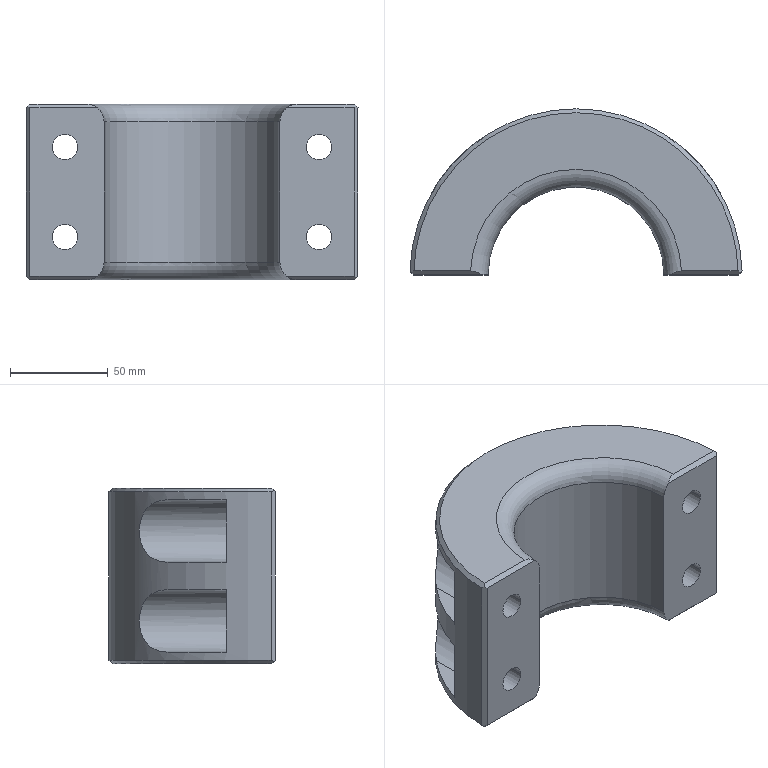Part | Creo | features DATUM PLANE 4, CURVE 3, CUT 2, CHAMFER 1, COORDINATE SYSTEM 1, PROTRUSION 1, ROUND 1 | 1 solid | 40 faces | box 170 x 85 x 90 mm | volume 620159 mm3 | plane 22 | cylinder 14 | torus 2 | cone 2 | commonest cylinder face diameters 13 x8 32 x4 90 x1 170 x1
STEP:
#1=CARTESIAN_POINT('',(0.,0.,0.));
#2=DIRECTION('',(0.,0.,1.));
#3=DIRECTION('',(1.,0.,0.));
#4=AXIS2_PLACEMENT_3D('',#1,#2,#3);
#5=CARTESIAN_POINT('',(53.963,2.,-45.));
#6=VERTEX_POINT('',#5);
#7=CARTESIAN_POINT('',(-53.963,2.,-45.));
#8=VERTEX_POINT('',#7);
#9=CARTESIAN_POINT('',(0.,0.,-45.));
#10=DIRECTION('',(0.,0.,1.));
#11=DIRECTION('',(0.9993,0.03704,0.));
#12=AXIS2_PLACEMENT_3D('',#9,#10,#11);
#13=CIRCLE('',#12,54.);
#14=EDGE_CURVE('',#6,#8,#13,.T.);
#15=ORIENTED_EDGE('',*,*,#14,.F.);
#16=CARTESIAN_POINT('',(82.976,2.,-45.));
#17=VERTEX_POINT('',#16);
#18=CARTESIAN_POINT('',(82.976,2.,-45.));
#19=DIRECTION('',(-1.,0.,-0.000000001));
#20=VECTOR('',#19,29.013);
#21=LINE('',#18,#20);
#22=EDGE_CURVE('',#17,#6,#21,.T.);
#23=ORIENTED_EDGE('',*,*,#22,.F.);
#24=CARTESIAN_POINT('',(-82.976,2.,-45.));
#25=VERTEX_POINT('',#24);
#26=CARTESIAN_POINT('',(-0.00000004,0.000000008,-45.));
#27=DIRECTION('',(0.,0.,-1.));
#28=DIRECTION('',(-0.9997,0.0241,0.));
#29=AXIS2_PLACEMENT_3D('',#26,#27,#28);
#30=CIRCLE('',#29,83.);
#31=EDGE_CURVE('',#25,#17,#30,.T.);
#32=ORIENTED_EDGE('',*,*,#31,.F.);
#33=CARTESIAN_POINT('',(-53.963,2.,-45.));
#34=DIRECTION('',(-1.,0.,0.));
#35=VECTOR('',#34,29.013);
#36=LINE('',#33,#35);
#37=EDGE_CURVE('',#8,#25,#36,.T.);
#38=ORIENTED_EDGE('',*,*,#37,.F.);
#39=EDGE_LOOP('',(#15,#23,#32,#38));
#40=FACE_OUTER_BOUND('',#39,.F.);
#41=CARTESIAN_POINT('',(0.,0.,-45.));
#42=DIRECTION('',(0.,0.,1.));
#43=DIRECTION('',(1.,0.,0.));
#44=AXIS2_PLACEMENT_3D('',#41,#42,#43);
#45=PLANE('',#44);
#46=ADVANCED_FACE('',(#40),#45,.F.);
#47=ORIENTED_EDGE('',*,*,#14,.T.);
#48=CARTESIAN_POINT('',(-48.343,0.,-43.));
#49=VERTEX_POINT('',#48);
#50=CARTESIAN_POINT('',(-53.546,2.,-45.));
#51=CARTESIAN_POINT('',(-52.717,1.945,-44.945));
#52=CARTESIAN_POINT('',(-51.42,1.663,-44.663));
#53=CARTESIAN_POINT('',(-50.257,1.222,-44.222));
#54=CARTESIAN_POINT('',(-49.214,0.653,-43.653));
#55=CARTESIAN_POINT('',(-48.622,0.2252,-43.225));
#56=B_SPLINE_CURVE_WITH_KNOTS('',3,(#7,#50,#51,#52,#53,#54,#55,#48),.UNSPECIFIED.,.F.,.F.,(4,1,1,1,1,4),(0.,0.2,0.4,0.6,0.8,1.),.UNSPECIFIED.);
#57=EDGE_CURVE('',#8,#49,#56,.T.);
#58=ORIENTED_EDGE('',*,*,#57,.T.);
#59=CARTESIAN_POINT('',(-45.,0.,-36.));
#60=VERTEX_POINT('',#59);
#61=CARTESIAN_POINT('',(-54.,0.,-36.));
#62=DIRECTION('',(0.,-1.,0.));
#63=DIRECTION('',(0.6285,0.,-0.7778));
#64=AXIS2_PLACEMENT_3D('',#61,#62,#63);
#65=CIRCLE('',#64,9.);
#66=EDGE_CURVE('',#49,#60,#65,.T.);
#67=ORIENTED_EDGE('',*,*,#66,.T.);
#68=CARTESIAN_POINT('',(45.,0.,-36.));
#69=VERTEX_POINT('',#68);
#70=CARTESIAN_POINT('',(0.,0.,-36.));
#71=DIRECTION('',(0.,0.,-1.));
#72=DIRECTION('',(-1.,0.,0.));
#73=AXIS2_PLACEMENT_3D('',#70,#71,#72);
#74=CIRCLE('',#73,45.);
#75=EDGE_CURVE('',#60,#69,#74,.T.);
#76=ORIENTED_EDGE('',*,*,#75,.T.);
#77=CARTESIAN_POINT('',(48.343,0.,-43.));
#78=VERTEX_POINT('',#77);
#79=CARTESIAN_POINT('',(54.,0.,-36.));
#80=DIRECTION('',(0.,-1.,0.));
#81=DIRECTION('',(-1.,0.,0.));
#82=AXIS2_PLACEMENT_3D('',#79,#80,#81);
#83=CIRCLE('',#82,9.);
#84=EDGE_CURVE('',#69,#78,#83,.T.);
#85=ORIENTED_EDGE('',*,*,#84,.T.);
#86=CARTESIAN_POINT('',(48.343,0.,-43.));
#87=CARTESIAN_POINT('',(48.622,0.2255,-43.226));
#88=CARTESIAN_POINT('',(49.215,0.6537,-43.654));
#89=CARTESIAN_POINT('',(50.258,1.222,-44.222));
#90=CARTESIAN_POINT('',(51.421,1.663,-44.663));
#91=CARTESIAN_POINT('',(52.717,1.945,-44.945));
#92=CARTESIAN_POINT('',(53.546,2.,-45.));
#93=B_SPLINE_CURVE_WITH_KNOTS('',3,(#86,#87,#88,#89,#90,#91,#92,#5),.UNSPECIFIED.,.F.,.F.,(4,1,1,1,1,4),(0.,0.2,0.4,0.6,0.8,1.),.UNSPECIFIED.);
#94=EDGE_CURVE('',#78,#6,#93,.T.);
#95=ORIENTED_EDGE('',*,*,#94,.T.);
#96=EDGE_LOOP('',(#47,#58,#67,#76,#85,#95));
#97=FACE_OUTER_BOUND('',#96,.F.);
#98=CARTESIAN_POINT('',(0.,0.,-36.));
#99=DIRECTION('',(0.,0.,1.));
#100=DIRECTION('',(0.001486,-1.,0.));
#101=AXIS2_PLACEMENT_3D('',#98,#99,#100);
#102=TOROIDAL_SURFACE('',#101,54.,9.);
#103=ADVANCED_FACE('',(#97),#102,.T.);
#104=ORIENTED_EDGE('',*,*,#57,.F.);
#105=ORIENTED_EDGE('',*,*,#37,.T.);
#106=CARTESIAN_POINT('',(-83.973,1.021,-44.021));
#107=VERTEX_POINT('',#106);
#108=CARTESIAN_POINT('',(-83.086,1.892,-44.892));
#109=CARTESIAN_POINT('',(-83.308,1.676,-44.676));
#110=CARTESIAN_POINT('',(-83.64,1.35,-44.35));
#111=CARTESIAN_POINT('',(-83.862,1.131,-44.131));
#112=CARTESIAN_POINT('',(-83.973,1.021,-44.021));
#113=B_SPLINE_CURVE_WITH_KNOTS('',3,(#24,#108,#109,#110,#111,#112),.UNSPECIFIED.,.F.,.F.,(4,1,1,4),(0.,0.3333,0.6667,1.),.UNSPECIFIED.);
#114=EDGE_CURVE('',#25,#107,#113,.T.);
#115=ORIENTED_EDGE('',*,*,#114,.T.);
#116=CARTESIAN_POINT('',(-82.976,0.,-43.));
#117=VERTEX_POINT('',#116);
#118=CARTESIAN_POINT('',(-83.973,1.021,-44.021));
#119=DIRECTION('',(0.5681,-0.5819,0.5819));
#120=VECTOR('',#119,1.755);
#121=LINE('',#118,#120);
#122=EDGE_CURVE('',#107,#117,#121,.T.);
#123=ORIENTED_EDGE('',*,*,#122,.T.);
#124=CARTESIAN_POINT('',(-48.343,0.,-43.));
#125=DIRECTION('',(-1.,0.,0.));
#126=VECTOR('',#125,34.633);
#127=LINE('',#124,#126);
#128=EDGE_CURVE('',#49,#117,#127,.T.);
#129=ORIENTED_EDGE('',*,*,#128,.F.);
#130=EDGE_LOOP('',(#104,#105,#115,#123,#129));
#131=FACE_OUTER_BOUND('',#130,.F.);
#132=CARTESIAN_POINT('',(-64.988,1.,-44.));
#133=DIRECTION('',(0.,-0.7071,-0.7071));
#134=DIRECTION('',(0.,-0.7071,0.7071));
#135=AXIS2_PLACEMENT_3D('',#132,#133,#134);
#136=PLANE('',#135);
#137=ADVANCED_FACE('',(#131),#136,.T.);
#138=ORIENTED_EDGE('',*,*,#31,.T.);
#139=CARTESIAN_POINT('',(83.973,1.021,-44.021));
#140=VERTEX_POINT('',#139);
#141=CARTESIAN_POINT('',(83.973,1.021,-44.021));
#142=CARTESIAN_POINT('',(83.862,1.131,-44.131));
#143=CARTESIAN_POINT('',(83.64,1.35,-44.35));
#144=CARTESIAN_POINT('',(83.308,1.676,-44.676));
#145=CARTESIAN_POINT('',(83.086,1.892,-44.892));
#146=B_SPLINE_CURVE_WITH_KNOTS('',3,(#141,#142,#143,#144,#145,#16),.UNSPECIFIED.,.F.,.F.,(4,1,1,4),(0.,0.3333,0.6667,1.),.UNSPECIFIED.);
#147=EDGE_CURVE('',#140,#17,#146,.T.);
#148=ORIENTED_EDGE('',*,*,#147,.F.);
#149=CARTESIAN_POINT('',(84.975,2.048,-43.));
#150=VERTEX_POINT('',#149);
#151=CARTESIAN_POINT('',(84.975,2.048,-43.));
#152=CARTESIAN_POINT('',(84.863,1.933,-43.115));
#153=CARTESIAN_POINT('',(84.639,1.704,-43.344));
#154=CARTESIAN_POINT('',(84.305,1.361,-43.684));
#155=CARTESIAN_POINT('',(84.083,1.134,-43.909));
#156=B_SPLINE_CURVE_WITH_KNOTS('',3,(#151,#152,#153,#154,#155,#139),.UNSPECIFIED.,.F.,.F.,(4,1,1,4),(0.,0.3333,0.6667,1.),.UNSPECIFIED.);
#157=EDGE_CURVE('',#150,#140,#156,.T.);
#158=ORIENTED_EDGE('',*,*,#157,.F.);
#159=CARTESIAN_POINT('',(-84.975,2.048,-43.));
#160=VERTEX_POINT('',#159);
#161=CARTESIAN_POINT('',(-0.00000004,0.000000008,-43.));
#162=DIRECTION('',(0.,0.,1.));
#163=DIRECTION('',(0.9997,0.0241,0.));
#164=AXIS2_PLACEMENT_3D('',#161,#162,#163);
#165=CIRCLE('',#164,85.);
#166=EDGE_CURVE('',#150,#160,#165,.T.);
#167=ORIENTED_EDGE('',*,*,#166,.T.);
#168=CARTESIAN_POINT('',(-84.975,2.048,-43.));
#169=CARTESIAN_POINT('',(-84.863,1.933,-43.115));
#170=CARTESIAN_POINT('',(-84.639,1.704,-43.344));
#171=CARTESIAN_POINT('',(-84.305,1.361,-43.684));
#172=CARTESIAN_POINT('',(-84.083,1.134,-43.909));
#173=B_SPLINE_CURVE_WITH_KNOTS('',3,(#168,#169,#170,#171,#172,#106),.UNSPECIFIED.,.F.,.F.,(4,1,1,4),(0.,0.3333,0.6667,1.),.UNSPECIFIED.);
#174=EDGE_CURVE('',#160,#107,#173,.T.);
#175=ORIENTED_EDGE('',*,*,#174,.T.);
#176=ORIENTED_EDGE('',*,*,#114,.F.);
#177=EDGE_LOOP('',(#138,#148,#158,#167,#175,#176));
#178=FACE_OUTER_BOUND('',#177,.F.);
#179=CARTESIAN_POINT('',(-0.00000004,0.000000008,-44.));
#180=DIRECTION('',(0.,0.,1.));
#181=DIRECTION('',(0.,-1.,0.));
#182=AXIS2_PLACEMENT_3D('',#179,#180,#181);
#183=CONICAL_SURFACE('',#182,84.,45.);
#184=ADVANCED_FACE('',(#178),#183,.T.);
#185=ORIENTED_EDGE('',*,*,#94,.F.);
#186=CARTESIAN_POINT('',(82.976,0.,-43.));
#187=VERTEX_POINT('',#186);
#188=CARTESIAN_POINT('',(82.976,0.,-43.));
#189=DIRECTION('',(-1.,0.,0.));
#190=VECTOR('',#189,34.633);
#191=LINE('',#188,#190);
#192=EDGE_CURVE('',#187,#78,#191,.T.);
#193=ORIENTED_EDGE('',*,*,#192,.F.);
#194=CARTESIAN_POINT('',(82.976,0.,-43.));
#195=DIRECTION('',(0.5681,0.5819,-0.5819));
#196=VECTOR('',#195,1.755);
#197=LINE('',#194,#196);
#198=EDGE_CURVE('',#187,#140,#197,.T.);
#199=ORIENTED_EDGE('',*,*,#198,.T.);
#200=ORIENTED_EDGE('',*,*,#147,.T.);
#201=ORIENTED_EDGE('',*,*,#22,.T.);
#202=EDGE_LOOP('',(#185,#193,#199,#200,#201));
#203=FACE_OUTER_BOUND('',#202,.F.);
#204=CARTESIAN_POINT('',(64.988,1.,-44.));
#205=DIRECTION('',(0.,-0.7071,-0.7071));
#206=DIRECTION('',(0.,-0.7071,0.7071));
#207=AXIS2_PLACEMENT_3D('',#204,#205,#206);
#208=PLANE('',#207);
#209=ADVANCED_FACE('',(#203),#208,.T.);
#210=ORIENTED_EDGE('',*,*,#84,.F.);
#211=CARTESIAN_POINT('',(45.,0.,36.));
#212=VERTEX_POINT('',#211);
#213=CARTESIAN_POINT('',(45.,0.,-36.));
#214=DIRECTION('',(0.,0.,1.));
#215=VECTOR('',#214,72.);
#216=LINE('',#213,#215);
#217=EDGE_CURVE('',#69,#212,#216,.T.);
#218=ORIENTED_EDGE('',*,*,#217,.T.);
#219=CARTESIAN_POINT('',(48.343,0.,43.));
#220=VERTEX_POINT('',#219);
#221=CARTESIAN_POINT('',(54.,0.,36.));
#222=DIRECTION('',(0.,-1.,0.));
#223=DIRECTION('',(-0.6285,0.,0.7778));
#224=AXIS2_PLACEMENT_3D('',#221,#222,#223);
#225=CIRCLE('',#224,9.);
#226=EDGE_CURVE('',#220,#212,#225,.T.);
#227=ORIENTED_EDGE('',*,*,#226,.F.);
#228=CARTESIAN_POINT('',(82.976,0.,43.));
#229=VERTEX_POINT('',#228);
#230=CARTESIAN_POINT('',(48.343,0.,43.));
#231=DIRECTION('',(1.,0.,0.));
#232=VECTOR('',#231,34.633);
#233=LINE('',#230,#232);
#234=EDGE_CURVE('',#220,#229,#233,.T.);
#235=ORIENTED_EDGE('',*,*,#234,.T.);
#236=CARTESIAN_POINT('',(82.976,0.,43.));
#237=DIRECTION('',(0.,0.,-1.));
#238=VECTOR('',#237,86.);
#239=LINE('',#236,#238);
#240=EDGE_CURVE('',#229,#187,#239,.T.);
#241=ORIENTED_EDGE('',*,*,#240,.T.);
#242=ORIENTED_EDGE('',*,*,#192,.T.);
#243=EDGE_LOOP('',(#210,#218,#227,#235,#241,#242));
#244=FACE_OUTER_BOUND('',#243,.F.);
#245=CARTESIAN_POINT('',(71.5,0.,23.));
#246=VERTEX_POINT('',#245);
#247=CARTESIAN_POINT('',(58.5,0.,23.));
#248=VERTEX_POINT('',#247);
#249=CARTESIAN_POINT('',(65.,0.,23.));
#250=DIRECTION('',(0.,1.,0.));
#251=DIRECTION('',(1.,0.,0.));
#252=AXIS2_PLACEMENT_3D('',#249,#250,#251);
#253=CIRCLE('',#252,6.5);
#254=EDGE_CURVE('',#246,#248,#253,.T.);
#255=ORIENTED_EDGE('',*,*,#254,.F.);
#256=CARTESIAN_POINT('',(65.,0.,23.));
#257=DIRECTION('',(0.,1.,0.));
#258=DIRECTION('',(-1.,0.,0.));
#259=AXIS2_PLACEMENT_3D('',#256,#257,#258);
#260=CIRCLE('',#259,6.5);
#261=EDGE_CURVE('',#248,#246,#260,.T.);
#262=ORIENTED_EDGE('',*,*,#261,.F.);
#263=EDGE_LOOP('',(#255,#262));
#264=FACE_BOUND('',#263,.F.);
#265=CARTESIAN_POINT('',(71.5,0.,-23.));
#266=VERTEX_POINT('',#265);
#267=CARTESIAN_POINT('',(58.5,0.,-23.));
#268=VERTEX_POINT('',#267);
#269=CARTESIAN_POINT('',(65.,0.,-23.));
#270=DIRECTION('',(0.,1.,0.));
#271=DIRECTION('',(1.,0.,0.));
#272=AXIS2_PLACEMENT_3D('',#269,#270,#271);
#273=CIRCLE('',#272,6.5);
#274=EDGE_CURVE('',#266,#268,#273,.T.);
#275=ORIENTED_EDGE('',*,*,#274,.F.);
#276=CARTESIAN_POINT('',(65.,0.,-23.));
#277=DIRECTION('',(0.,1.,0.));
#278=DIRECTION('',(-1.,0.,0.));
#279=AXIS2_PLACEMENT_3D('',#276,#277,#278);
#280=CIRCLE('',#279,6.5);
#281=EDGE_CURVE('',#268,#266,#280,.T.);
#282=ORIENTED_EDGE('',*,*,#281,.F.);
#283=EDGE_LOOP('',(#275,#282));
#284=FACE_BOUND('',#283,.F.);
#285=CARTESIAN_POINT('',(45.,0.,-45.));
#286=DIRECTION('',(0.,-1.,0.));
#287=DIRECTION('',(1.,0.,0.));
#288=AXIS2_PLACEMENT_3D('',#285,#286,#287);
#289=PLANE('',#288);
#290=ADVANCED_FACE('',(#244,#264,#284),#289,.T.);
#291=ORIENTED_EDGE('',*,*,#274,.T.);
#292=CARTESIAN_POINT('',(58.5,25.,-23.));
#293=VERTEX_POINT('',#292);
#294=CARTESIAN_POINT('',(58.5,25.,-23.));
#295=DIRECTION('',(0.,-1.,0.));
#296=VECTOR('',#295,25.);
#297=LINE('',#294,#296);
#298=EDGE_CURVE('',#293,#268,#297,.T.);
#299=ORIENTED_EDGE('',*,*,#298,.F.);
#300=CARTESIAN_POINT('',(71.5,25.,-23.));
#301=VERTEX_POINT('',#300);
#302=CARTESIAN_POINT('',(65.,25.,-23.));
#303=DIRECTION('',(0.,1.,0.));
#304=DIRECTION('',(1.,0.,0.));
#305=AXIS2_PLACEMENT_3D('',#302,#303,#304);
#306=CIRCLE('',#305,6.5);
#307=EDGE_CURVE('',#301,#293,#306,.T.);
#308=ORIENTED_EDGE('',*,*,#307,.F.);
#309=CARTESIAN_POINT('',(71.5,25.,-23.));
#310=DIRECTION('',(0.,-1.,0.));
#311=VECTOR('',#310,25.);
#312=LINE('',#309,#311);
#313=EDGE_CURVE('',#301,#266,#312,.T.);
#314=ORIENTED_EDGE('',*,*,#313,.T.);
#315=EDGE_LOOP('',(#291,#299,#308,#314));
#316=FACE_OUTER_BOUND('',#315,.F.);
#317=CARTESIAN_POINT('',(65.,25.,-23.));
#318=DIRECTION('',(0.,1.,0.));
#319=DIRECTION('',(1.,0.,0.));
#320=AXIS2_PLACEMENT_3D('',#317,#318,#319);
#321=CYLINDRICAL_SURFACE('',#320,6.5);
#322=ADVANCED_FACE('',(#316),#321,.F.);
#323=ORIENTED_EDGE('',*,*,#281,.T.);
#324=ORIENTED_EDGE('',*,*,#313,.F.);
#325=CARTESIAN_POINT('',(65.,25.,-23.));
#326=DIRECTION('',(0.,1.,0.));
#327=DIRECTION('',(-1.,0.,0.));
#328=AXIS2_PLACEMENT_3D('',#325,#326,#327);
#329=CIRCLE('',#328,6.5);
#330=EDGE_CURVE('',#293,#301,#329,.T.);
#331=ORIENTED_EDGE('',*,*,#330,.F.);
#332=ORIENTED_EDGE('',*,*,#298,.T.);
#333=EDGE_LOOP('',(#323,#324,#331,#332));
#334=FACE_OUTER_BOUND('',#333,.F.);
#335=CARTESIAN_POINT('',(65.,25.,-23.));
#336=DIRECTION('',(0.,1.,0.));
#337=DIRECTION('',(1.,0.,0.));
#338=AXIS2_PLACEMENT_3D('',#335,#336,#337);
#339=CYLINDRICAL_SURFACE('',#338,6.5);
#340=ADVANCED_FACE('',(#334),#339,.F.);
#341=CARTESIAN_POINT('',(81.24,25.,-39.));
#342=VERTEX_POINT('',#341);
#343=CARTESIAN_POINT('',(81.24,25.,-7.));
#344=VERTEX_POINT('',#343);
#345=CARTESIAN_POINT('',(81.24,25.,-39.));
#346=DIRECTION('',(0.,0.,1.));
#347=VECTOR('',#346,32.);
#348=LINE('',#345,#347);
#349=EDGE_CURVE('',#342,#344,#348,.T.);
#350=ORIENTED_EDGE('',*,*,#349,.T.);
#351=CARTESIAN_POINT('',(65.,25.,-7.));
#352=VERTEX_POINT('',#351);
#353=CARTESIAN_POINT('',(65.,25.,-7.));
#354=DIRECTION('',(1.,0.,0.));
#355=VECTOR('',#354,16.24);
#356=LINE('',#353,#355);
#357=EDGE_CURVE('',#352,#344,#356,.T.);
#358=ORIENTED_EDGE('',*,*,#357,.F.);
#359=CARTESIAN_POINT('',(65.,25.,-39.));
#360=VERTEX_POINT('',#359);
#361=CARTESIAN_POINT('',(65.,25.,-23.));
#362=DIRECTION('',(0.,1.,0.));
#363=DIRECTION('',(0.,0.,-1.));
#364=AXIS2_PLACEMENT_3D('',#361,#362,#363);
#365=CIRCLE('',#364,16.);
#366=EDGE_CURVE('',#360,#352,#365,.T.);
#367=ORIENTED_EDGE('',*,*,#366,.F.);
#368=CARTESIAN_POINT('',(81.24,25.,-39.));
#369=DIRECTION('',(-1.,0.,0.));
#370=VECTOR('',#369,16.24);
#371=LINE('',#368,#370);
#372=EDGE_CURVE('',#342,#360,#371,.T.);
#373=ORIENTED_EDGE('',*,*,#372,.F.);
#374=EDGE_LOOP('',(#350,#358,#367,#373));
#375=FACE_OUTER_BOUND('',#374,.F.);
#376=ORIENTED_EDGE('',*,*,#307,.T.);
#377=ORIENTED_EDGE('',*,*,#330,.T.);
#378=EDGE_LOOP('',(#376,#377));
#379=FACE_BOUND('',#378,.F.);
#380=CARTESIAN_POINT('',(0.,25.,0.));
#381=DIRECTION('',(0.,1.,0.));
#382=DIRECTION('',(1.,0.,0.));
#383=AXIS2_PLACEMENT_3D('',#380,#381,#382);
#384=PLANE('',#383);
#385=ADVANCED_FACE('',(#375,#379),#384,.T.);
#386=CARTESIAN_POINT('',(81.24,25.,7.));
#387=VERTEX_POINT('',#386);
#388=CARTESIAN_POINT('',(81.24,25.,39.));
#389=VERTEX_POINT('',#388);
#390=CARTESIAN_POINT('',(81.24,25.,7.));
#391=DIRECTION('',(0.,0.,1.));
#392=VECTOR('',#391,32.);
#393=LINE('',#390,#392);
#394=EDGE_CURVE('',#387,#389,#393,.T.);
#395=ORIENTED_EDGE('',*,*,#394,.T.);
#396=CARTESIAN_POINT('',(65.,25.,39.));
#397=VERTEX_POINT('',#396);
#398=CARTESIAN_POINT('',(65.,25.,39.));
#399=DIRECTION('',(1.,0.,0.));
#400=VECTOR('',#399,16.24);
#401=LINE('',#398,#400);
#402=EDGE_CURVE('',#397,#389,#401,.T.);
#403=ORIENTED_EDGE('',*,*,#402,.F.);
#404=CARTESIAN_POINT('',(65.,25.,7.));
#405=VERTEX_POINT('',#404);
#406=CARTESIAN_POINT('',(65.,25.,23.));
#407=DIRECTION('',(0.,1.,0.));
#408=DIRECTION('',(0.,0.,-1.));
#409=AXIS2_PLACEMENT_3D('',#406,#407,#408);
#410=CIRCLE('',#409,16.);
#411=EDGE_CURVE('',#405,#397,#410,.T.);
#412=ORIENTED_EDGE('',*,*,#411,.F.);
#413=CARTESIAN_POINT('',(81.24,25.,7.));
#414=DIRECTION('',(-1.,0.,0.));
#415=VECTOR('',#414,16.24);
#416=LINE('',#413,#415);
#417=EDGE_CURVE('',#387,#405,#416,.T.);
#418=ORIENTED_EDGE('',*,*,#417,.F.);
#419=EDGE_LOOP('',(#395,#403,#412,#418));
#420=FACE_OUTER_BOUND('',#419,.F.);
#421=CARTESIAN_POINT('',(71.5,25.,23.));
#422=VERTEX_POINT('',#421);
#423=CARTESIAN_POINT('',(58.5,25.,23.));
#424=VERTEX_POINT('',#423);
#425=CARTESIAN_POINT('',(65.,25.,23.));
#426=DIRECTION('',(0.,1.,0.));
#427=DIRECTION('',(1.,0.,0.));
#428=AXIS2_PLACEMENT_3D('',#425,#426,#427);
#429=CIRCLE('',#428,6.5);
#430=EDGE_CURVE('',#422,#424,#429,.T.);
#431=ORIENTED_EDGE('',*,*,#430,.T.);
#432=CARTESIAN_POINT('',(65.,25.,23.));
#433=DIRECTION('',(0.,1.,0.));
#434=DIRECTION('',(-1.,0.,0.));
#435=AXIS2_PLACEMENT_3D('',#432,#433,#434);
#436=CIRCLE('',#435,6.5);
#437=EDGE_CURVE('',#424,#422,#436,.T.);
#438=ORIENTED_EDGE('',*,*,#437,.T.);
#439=EDGE_LOOP('',(#431,#438));
#440=FACE_BOUND('',#439,.F.);
#441=CARTESIAN_POINT('',(0.,25.,0.));
#442=DIRECTION('',(0.,1.,0.));
#443=DIRECTION('',(1.,0.,0.));
#444=AXIS2_PLACEMENT_3D('',#441,#442,#443);
#445=PLANE('',#444);
#446=ADVANCED_FACE('',(#420,#440),#445,.T.);
#447=CARTESIAN_POINT('',(-81.24,25.,-39.));
#448=VERTEX_POINT('',#447);
#449=CARTESIAN_POINT('',(-81.24,25.,-7.));
#450=VERTEX_POINT('',#449);
#451=CARTESIAN_POINT('',(-81.24,25.,-39.));
#452=DIRECTION('',(0.,0.,1.));
#453=VECTOR('',#452,32.);
#454=LINE('',#451,#453);
#455=EDGE_CURVE('',#448,#450,#454,.T.);
#456=ORIENTED_EDGE('',*,*,#455,.F.);
#457=CARTESIAN_POINT('',(-65.,25.,-39.));
#458=VERTEX_POINT('',#457);
#459=CARTESIAN_POINT('',(-65.,25.,-39.));
#460=DIRECTION('',(-1.,0.,0.));
#461=VECTOR('',#460,16.24);
#462=LINE('',#459,#461);
#463=EDGE_CURVE('',#458,#448,#462,.T.);
#464=ORIENTED_EDGE('',*,*,#463,.F.);
#465=CARTESIAN_POINT('',(-65.,25.,-7.));
#466=VERTEX_POINT('',#465);
#467=CARTESIAN_POINT('',(-65.,25.,-23.));
#468=DIRECTION('',(0.,1.,0.));
#469=DIRECTION('',(0.,0.,1.));
#470=AXIS2_PLACEMENT_3D('',#467,#468,#469);
#471=CIRCLE('',#470,16.);
#472=EDGE_CURVE('',#466,#458,#471,.T.);
#473=ORIENTED_EDGE('',*,*,#472,.F.);
#474=CARTESIAN_POINT('',(-81.24,25.,-7.));
#475=DIRECTION('',(1.,0.,0.));
#476=VECTOR('',#475,16.24);
#477=LINE('',#474,#476);
#478=EDGE_CURVE('',#450,#466,#477,.T.);
#479=ORIENTED_EDGE('',*,*,#478,.F.);
#480=EDGE_LOOP('',(#456,#464,#473,#479));
#481=FACE_OUTER_BOUND('',#480,.F.);
#482=CARTESIAN_POINT('',(-58.5,25.,-23.));
#483=VERTEX_POINT('',#482);
#484=CARTESIAN_POINT('',(-71.5,25.,-23.));
#485=VERTEX_POINT('',#484);
#486=CARTESIAN_POINT('',(-65.,25.,-23.));
#487=DIRECTION('',(0.,1.,0.));
#488=DIRECTION('',(1.,0.,0.));
#489=AXIS2_PLACEMENT_3D('',#486,#487,#488);
#490=CIRCLE('',#489,6.5);
#491=EDGE_CURVE('',#483,#485,#490,.T.);
#492=ORIENTED_EDGE('',*,*,#491,.T.);
#493=CARTESIAN_POINT('',(-65.,25.,-23.));
#494=DIRECTION('',(0.,1.,0.));
#495=DIRECTION('',(-1.,0.,0.));
#496=AXIS2_PLACEMENT_3D('',#493,#494,#495);
#497=CIRCLE('',#496,6.5);
#498=EDGE_CURVE('',#485,#483,#497,.T.);
#499=ORIENTED_EDGE('',*,*,#498,.T.);
#500=EDGE_LOOP('',(#492,#499));
#501=FACE_BOUND('',#500,.F.);
#502=CARTESIAN_POINT('',(0.,25.,0.));
#503=DIRECTION('',(0.,1.,0.));
#504=DIRECTION('',(1.,0.,0.));
#505=AXIS2_PLACEMENT_3D('',#502,#503,#504);
#506=PLANE('',#505);
#507=ADVANCED_FACE('',(#481,#501),#506,.T.);
#508=CARTESIAN_POINT('',(-81.24,25.,7.));
#509=VERTEX_POINT('',#508);
#510=CARTESIAN_POINT('',(-81.24,25.,39.));
#511=VERTEX_POINT('',#510);
#512=CARTESIAN_POINT('',(-81.24,25.,7.));
#513=DIRECTION('',(0.,0.,1.));
#514=VECTOR('',#513,32.);
#515=LINE('',#512,#514);
#516=EDGE_CURVE('',#509,#511,#515,.T.);
#517=ORIENTED_EDGE('',*,*,#516,.F.);
#518=CARTESIAN_POINT('',(-65.,25.,7.));
#519=VERTEX_POINT('',#518);
#520=CARTESIAN_POINT('',(-65.,25.,7.));
#521=DIRECTION('',(-1.,0.,0.));
#522=VECTOR('',#521,16.24);
#523=LINE('',#520,#522);
#524=EDGE_CURVE('',#519,#509,#523,.T.);
#525=ORIENTED_EDGE('',*,*,#524,.F.);
#526=CARTESIAN_POINT('',(-65.,25.,39.));
#527=VERTEX_POINT('',#526);
#528=CARTESIAN_POINT('',(-65.,25.,23.));
#529=DIRECTION('',(0.,1.,0.));
#530=DIRECTION('',(0.,0.,1.));
#531=AXIS2_PLACEMENT_3D('',#528,#529,#530);
#532=CIRCLE('',#531,16.);
#533=EDGE_CURVE('',#527,#519,#532,.T.);
#534=ORIENTED_EDGE('',*,*,#533,.F.);
#535=CARTESIAN_POINT('',(-81.24,25.,39.));
#536=DIRECTION('',(1.,0.,0.));
#537=VECTOR('',#536,16.24);
#538=LINE('',#535,#537);
#539=EDGE_CURVE('',#511,#527,#538,.T.);
#540=ORIENTED_EDGE('',*,*,#539,.F.);
#541=EDGE_LOOP('',(#517,#525,#534,#540));
#542=FACE_OUTER_BOUND('',#541,.F.);
#543=CARTESIAN_POINT('',(-58.5,25.,23.));
#544=VERTEX_POINT('',#543);
#545=CARTESIAN_POINT('',(-71.5,25.,23.));
#546=VERTEX_POINT('',#545);
#547=CARTESIAN_POINT('',(-65.,25.,23.));
#548=DIRECTION('',(0.,1.,0.));
#549=DIRECTION('',(1.,0.,0.));
#550=AXIS2_PLACEMENT_3D('',#547,#548,#549);
#551=CIRCLE('',#550,6.5);
#552=EDGE_CURVE('',#544,#546,#551,.T.);
#553=ORIENTED_EDGE('',*,*,#552,.T.);
#554=CARTESIAN_POINT('',(-65.,25.,23.));
#555=DIRECTION('',(0.,1.,0.));
#556=DIRECTION('',(-1.,0.,0.));
#557=AXIS2_PLACEMENT_3D('',#554,#555,#556);
#558=CIRCLE('',#557,6.5);
#559=EDGE_CURVE('',#546,#544,#558,.T.);
#560=ORIENTED_EDGE('',*,*,#559,.T.);
#561=EDGE_LOOP('',(#553,#560));
#562=FACE_BOUND('',#561,.F.);
#563=CARTESIAN_POINT('',(0.,25.,0.));
#564=DIRECTION('',(0.,1.,0.));
#565=DIRECTION('',(1.,0.,0.));
#566=AXIS2_PLACEMENT_3D('',#563,#564,#565);
#567=PLANE('',#566);
#568=ADVANCED_FACE('',(#542,#562),#567,.T.);
#569=CARTESIAN_POINT('',(-84.975,2.048,43.));
#570=VERTEX_POINT('',#569);
#571=CARTESIAN_POINT('',(-84.975,2.048,43.));
#572=DIRECTION('',(0.,0.,-1.));
#573=VECTOR('',#572,86.);
#574=LINE('',#571,#573);
#575=EDGE_CURVE('',#570,#160,#574,.T.);
#576=ORIENTED_EDGE('',*,*,#575,.T.);
#577=ORIENTED_EDGE('',*,*,#166,.F.);
#578=CARTESIAN_POINT('',(84.975,2.048,43.));
#579=VERTEX_POINT('',#578);
#580=CARTESIAN_POINT('',(84.975,2.048,43.));
#581=DIRECTION('',(0.,0.,-1.));
#582=VECTOR('',#581,86.);
#583=LINE('',#580,#582);
#584=EDGE_CURVE('',#579,#150,#583,.T.);
#585=ORIENTED_EDGE('',*,*,#584,.F.);
#586=CARTESIAN_POINT('',(-0.00000004,-0.000000008,43.));
#587=DIRECTION('',(0.,0.,-1.));
#588=DIRECTION('',(-0.9997,0.0241,0.));
#589=AXIS2_PLACEMENT_3D('',#586,#587,#588);
#590=CIRCLE('',#589,85.);
#591=EDGE_CURVE('',#570,#579,#590,.T.);
#592=ORIENTED_EDGE('',*,*,#591,.F.);
#593=EDGE_LOOP('',(#576,#577,#585,#592));
#594=FACE_OUTER_BOUND('',#593,.F.);
#595=ORIENTED_EDGE('',*,*,#394,.F.);
#596=CARTESIAN_POINT('',(65.,54.772,7.));
#597=VERTEX_POINT('',#596);
#598=CARTESIAN_POINT('',(0.,0.,7.));
#599=DIRECTION('',(0.,0.,1.));
#600=DIRECTION('',(0.9558,0.2941,0.));
#601=AXIS2_PLACEMENT_3D('',#598,#599,#600);
#602=CIRCLE('',#601,85.);
#603=EDGE_CURVE('',#387,#597,#602,.T.);
#604=ORIENTED_EDGE('',*,*,#603,.T.);
#605=CARTESIAN_POINT('',(65.,54.772,39.));
#606=VERTEX_POINT('',#605);
#607=CARTESIAN_POINT('',(64.503,55.362,39.));
#608=CARTESIAN_POINT('',(63.497,56.524,38.954));
#609=CARTESIAN_POINT('',(61.952,58.213,38.734));
#610=CARTESIAN_POINT('',(60.373,59.848,38.346));
#611=CARTESIAN_POINT('',(58.77,61.423,37.772));
#612=CARTESIAN_POINT('',(57.116,62.965,36.967));
#613=CARTESIAN_POINT('',(55.393,64.486,35.855));
#614=CARTESIAN_POINT('',(53.621,65.967,34.342));
#615=CARTESIAN_POINT('',(51.85,67.365,32.264));
#616=CARTESIAN_POINT('',(50.391,68.458,29.734));
#617=CARTESIAN_POINT('',(49.44,69.144,27.065));
#618=CARTESIAN_POINT('',(48.974,69.474,24.297));
#619=CARTESIAN_POINT('',(48.985,69.466,21.573));
#620=CARTESIAN_POINT('',(49.474,69.12,18.805));
#621=CARTESIAN_POINT('',(50.449,68.416,16.141));
#622=CARTESIAN_POINT('',(51.927,67.305,13.628));
#623=CARTESIAN_POINT('',(53.694,65.907,11.588));
#624=CARTESIAN_POINT('',(55.446,64.44,10.107));
#625=CARTESIAN_POINT('',(57.153,62.93,9.012));
#626=CARTESIAN_POINT('',(58.794,61.4,8.218));
#627=CARTESIAN_POINT('',(60.388,59.832,7.649));
#628=CARTESIAN_POINT('',(61.962,58.202,7.264));
#629=CARTESIAN_POINT('',(63.501,56.519,7.046));
#630=CARTESIAN_POINT('',(64.504,55.36,7.));
#631=CARTESIAN_POINT('',(65.,54.772,7.));
#632=B_SPLINE_CURVE_WITH_KNOTS('',3,(#605,#607,#608,#609,#610,#611,#612,#613,#614,#615,#616,#617,#618,#619,#620,#621,#622,#623,#624,#625,#626,#627,#628,#629,#630,#631),.UNSPECIFIED.,.F.,.F.,(4,1,1,1,1,1,1,1,1,1,1,1,1,1,1,1,1,1,1,1,1,1,1,4),(0.,0.04348,0.08696,0.1304,0.1739,0.2174,0.2609,0.3043,0.3478,0.3913,0.4348,0.4783,0.5217,0.5652,0.6087,0.6522,0.6957,0.7391,0.7826,0.8261,0.8696,0.913,0.9565,1.),.UNSPECIFIED.);
#633=EDGE_CURVE('',#606,#597,#632,.T.);
#634=ORIENTED_EDGE('',*,*,#633,.F.);
#635=CARTESIAN_POINT('',(0.,0.,39.));
#636=DIRECTION('',(0.,0.,1.));
#637=DIRECTION('',(0.9558,0.2941,0.));
#638=AXIS2_PLACEMENT_3D('',#635,#636,#637);
#639=CIRCLE('',#638,85.);
#640=EDGE_CURVE('',#389,#606,#639,.T.);
#641=ORIENTED_EDGE('',*,*,#640,.F.);
#642=EDGE_LOOP('',(#595,#604,#634,#641));
#643=FACE_BOUND('',#642,.F.);
#644=ORIENTED_EDGE('',*,*,#455,.T.);
#645=CARTESIAN_POINT('',(-65.,54.772,-7.));
#646=VERTEX_POINT('',#645);
#647=CARTESIAN_POINT('',(0.,0.,-7.));
#648=DIRECTION('',(0.,0.,1.));
#649=DIRECTION('',(-0.7647,0.6444,0.));
#650=AXIS2_PLACEMENT_3D('',#647,#648,#649);
#651=CIRCLE('',#650,85.);
#652=EDGE_CURVE('',#646,#450,#651,.T.);
#653=ORIENTED_EDGE('',*,*,#652,.F.);
#654=CARTESIAN_POINT('',(-65.,54.772,-39.));
#655=VERTEX_POINT('',#654);
#656=CARTESIAN_POINT('',(-64.503,55.362,-39.));
#657=CARTESIAN_POINT('',(-63.497,56.524,-38.954));
#658=CARTESIAN_POINT('',(-61.952,58.213,-38.734));
#659=CARTESIAN_POINT('',(-60.373,59.848,-38.346));
#660=CARTESIAN_POINT('',(-58.77,61.423,-37.772));
#661=CARTESIAN_POINT('',(-57.116,62.965,-36.967));
#662=CARTESIAN_POINT('',(-55.393,64.486,-35.855));
#663=CARTESIAN_POINT('',(-53.621,65.967,-34.342));
#664=CARTESIAN_POINT('',(-51.85,67.365,-32.264));
#665=CARTESIAN_POINT('',(-50.391,68.458,-29.734));
#666=CARTESIAN_POINT('',(-49.44,69.144,-27.065));
#667=CARTESIAN_POINT('',(-48.974,69.474,-24.297));
#668=CARTESIAN_POINT('',(-48.985,69.466,-21.573));
#669=CARTESIAN_POINT('',(-49.474,69.12,-18.805));
#670=CARTESIAN_POINT('',(-50.449,68.416,-16.141));
#671=CARTESIAN_POINT('',(-51.927,67.305,-13.628));
#672=CARTESIAN_POINT('',(-53.694,65.907,-11.588));
#673=CARTESIAN_POINT('',(-55.446,64.44,-10.107));
#674=CARTESIAN_POINT('',(-57.153,62.93,-9.012));
#675=CARTESIAN_POINT('',(-58.794,61.4,-8.218));
#676=CARTESIAN_POINT('',(-60.388,59.832,-7.649));
#677=CARTESIAN_POINT('',(-61.962,58.202,-7.264));
#678=CARTESIAN_POINT('',(-63.501,56.519,-7.046));
#679=CARTESIAN_POINT('',(-64.504,55.36,-7.));
#680=CARTESIAN_POINT('',(-65.,54.772,-7.));
#681=B_SPLINE_CURVE_WITH_KNOTS('',3,(#654,#656,#657,#658,#659,#660,#661,#662,#663,#664,#665,#666,#667,#668,#669,#670,#671,#672,#673,#674,#675,#676,#677,#678,#679,#680),.UNSPECIFIED.,.F.,.F.,(4,1,1,1,1,1,1,1,1,1,1,1,1,1,1,1,1,1,1,1,1,1,1,4),(0.,0.04348,0.08696,0.1304,0.1739,0.2174,0.2609,0.3043,0.3478,0.3913,0.4348,0.4783,0.5217,0.5652,0.6087,0.6522,0.6957,0.7391,0.7826,0.8261,0.8696,0.913,0.9565,1.),.UNSPECIFIED.);
#682=EDGE_CURVE('',#655,#646,#681,.T.);
#683=ORIENTED_EDGE('',*,*,#682,.F.);
#684=CARTESIAN_POINT('',(0.,0.,-39.));
#685=DIRECTION('',(0.,0.,1.));
#686=DIRECTION('',(-0.7647,0.6444,0.));
#687=AXIS2_PLACEMENT_3D('',#684,#685,#686);
#688=CIRCLE('',#687,85.);
#689=EDGE_CURVE('',#655,#448,#688,.T.);
#690=ORIENTED_EDGE('',*,*,#689,.T.);
#691=EDGE_LOOP('',(#644,#653,#683,#690));
#692=FACE_BOUND('',#691,.F.);
#693=ORIENTED_EDGE('',*,*,#516,.T.);
#694=CARTESIAN_POINT('',(-65.,54.772,39.));
#695=VERTEX_POINT('',#694);
#696=CARTESIAN_POINT('',(0.,0.,39.));
#697=DIRECTION('',(0.,0.,1.));
#698=DIRECTION('',(-0.7647,0.6444,0.));
#699=AXIS2_PLACEMENT_3D('',#696,#697,#698);
#700=CIRCLE('',#699,85.);
#701=EDGE_CURVE('',#695,#511,#700,.T.);
#702=ORIENTED_EDGE('',*,*,#701,.F.);
#703=CARTESIAN_POINT('',(-65.,54.772,7.));
#704=VERTEX_POINT('',#703);
#705=CARTESIAN_POINT('',(-64.503,55.362,7.));
#706=CARTESIAN_POINT('',(-63.497,56.524,7.046));
#707=CARTESIAN_POINT('',(-61.952,58.213,7.266));
#708=CARTESIAN_POINT('',(-60.373,59.848,7.654));
#709=CARTESIAN_POINT('',(-58.77,61.423,8.228));
#710=CARTESIAN_POINT('',(-57.116,62.965,9.033));
#711=CARTESIAN_POINT('',(-55.393,64.486,10.145));
#712=CARTESIAN_POINT('',(-53.621,65.967,11.658));
#713=CARTESIAN_POINT('',(-51.85,67.365,13.736));
#714=CARTESIAN_POINT('',(-50.391,68.458,16.266));
#715=CARTESIAN_POINT('',(-49.44,69.144,18.935));
#716=CARTESIAN_POINT('',(-48.974,69.474,21.703));
#717=CARTESIAN_POINT('',(-48.985,69.466,24.427));
#718=CARTESIAN_POINT('',(-49.474,69.12,27.195));
#719=CARTESIAN_POINT('',(-50.449,68.416,29.859));
#720=CARTESIAN_POINT('',(-51.927,67.305,32.372));
#721=CARTESIAN_POINT('',(-53.694,65.907,34.412));
#722=CARTESIAN_POINT('',(-55.446,64.44,35.893));
#723=CARTESIAN_POINT('',(-57.153,62.93,36.988));
#724=CARTESIAN_POINT('',(-58.794,61.4,37.782));
#725=CARTESIAN_POINT('',(-60.388,59.832,38.351));
#726=CARTESIAN_POINT('',(-61.962,58.202,38.736));
#727=CARTESIAN_POINT('',(-63.501,56.519,38.954));
#728=CARTESIAN_POINT('',(-64.504,55.36,39.));
#729=CARTESIAN_POINT('',(-65.,54.772,39.));
#730=B_SPLINE_CURVE_WITH_KNOTS('',3,(#703,#705,#706,#707,#708,#709,#710,#711,#712,#713,#714,#715,#716,#717,#718,#719,#720,#721,#722,#723,#724,#725,#726,#727,#728,#729),.UNSPECIFIED.,.F.,.F.,(4,1,1,1,1,1,1,1,1,1,1,1,1,1,1,1,1,1,1,1,1,1,1,4),(0.,0.04348,0.08696,0.1304,0.1739,0.2174,0.2609,0.3043,0.3478,0.3913,0.4348,0.4783,0.5217,0.5652,0.6087,0.6522,0.6957,0.7391,0.7826,0.8261,0.8696,0.913,0.9565,1.),.UNSPECIFIED.);
#731=EDGE_CURVE('',#704,#695,#730,.T.);
#732=ORIENTED_EDGE('',*,*,#731,.F.);
#733=CARTESIAN_POINT('',(0.,0.,7.));
#734=DIRECTION('',(0.,0.,1.));
#735=DIRECTION('',(-0.7647,0.6444,0.));
#736=AXIS2_PLACEMENT_3D('',#733,#734,#735);
#737=CIRCLE('',#736,85.);
#738=EDGE_CURVE('',#704,#509,#737,.T.);
#739=ORIENTED_EDGE('',*,*,#738,.T.);
#740=EDGE_LOOP('',(#693,#702,#732,#739));
#741=FACE_BOUND('',#740,.F.);
#742=ORIENTED_EDGE('',*,*,#349,.F.);
#743=CARTESIAN_POINT('',(65.,54.772,-39.));
#744=VERTEX_POINT('',#743);
#745=CARTESIAN_POINT('',(0.,0.,-39.));
#746=DIRECTION('',(0.,0.,1.));
#747=DIRECTION('',(0.9558,0.2941,0.));
#748=AXIS2_PLACEMENT_3D('',#745,#746,#747);
#749=CIRCLE('',#748,85.);
#750=EDGE_CURVE('',#342,#744,#749,.T.);
#751=ORIENTED_EDGE('',*,*,#750,.T.);
#752=CARTESIAN_POINT('',(65.,54.772,-7.));
#753=VERTEX_POINT('',#752);
#754=CARTESIAN_POINT('',(64.503,55.362,-7.));
#755=CARTESIAN_POINT('',(63.497,56.524,-7.046));
#756=CARTESIAN_POINT('',(61.952,58.213,-7.266));
#757=CARTESIAN_POINT('',(60.373,59.848,-7.654));
#758=CARTESIAN_POINT('',(58.77,61.423,-8.228));
#759=CARTESIAN_POINT('',(57.116,62.965,-9.033));
#760=CARTESIAN_POINT('',(55.393,64.486,-10.145));
#761=CARTESIAN_POINT('',(53.621,65.967,-11.658));
#762=CARTESIAN_POINT('',(51.85,67.365,-13.736));
#763=CARTESIAN_POINT('',(50.391,68.458,-16.266));
#764=CARTESIAN_POINT('',(49.44,69.144,-18.935));
#765=CARTESIAN_POINT('',(48.974,69.474,-21.703));
#766=CARTESIAN_POINT('',(48.985,69.466,-24.427));
#767=CARTESIAN_POINT('',(49.474,69.12,-27.195));
#768=CARTESIAN_POINT('',(50.449,68.416,-29.859));
#769=CARTESIAN_POINT('',(51.927,67.305,-32.372));
#770=CARTESIAN_POINT('',(53.694,65.907,-34.412));
#771=CARTESIAN_POINT('',(55.446,64.44,-35.893));
#772=CARTESIAN_POINT('',(57.153,62.93,-36.988));
#773=CARTESIAN_POINT('',(58.794,61.4,-37.782));
#774=CARTESIAN_POINT('',(60.388,59.832,-38.351));
#775=CARTESIAN_POINT('',(61.962,58.202,-38.736));
#776=CARTESIAN_POINT('',(63.501,56.519,-38.954));
#777=CARTESIAN_POINT('',(64.504,55.36,-39.));
#778=CARTESIAN_POINT('',(65.,54.772,-39.));
#779=B_SPLINE_CURVE_WITH_KNOTS('',3,(#752,#754,#755,#756,#757,#758,#759,#760,#761,#762,#763,#764,#765,#766,#767,#768,#769,#770,#771,#772,#773,#774,#775,#776,#777,#778),.UNSPECIFIED.,.F.,.F.,(4,1,1,1,1,1,1,1,1,1,1,1,1,1,1,1,1,1,1,1,1,1,1,4),(0.,0.04348,0.08696,0.1304,0.1739,0.2174,0.2609,0.3043,0.3478,0.3913,0.4348,0.4783,0.5217,0.5652,0.6087,0.6522,0.6957,0.7391,0.7826,0.8261,0.8696,0.913,0.9565,1.),.UNSPECIFIED.);
#780=EDGE_CURVE('',#753,#744,#779,.T.);
#781=ORIENTED_EDGE('',*,*,#780,.F.);
#782=CARTESIAN_POINT('',(0.,0.,-7.));
#783=DIRECTION('',(0.,0.,1.));
#784=DIRECTION('',(0.9558,0.2941,0.));
#785=AXIS2_PLACEMENT_3D('',#782,#783,#784);
#786=CIRCLE('',#785,85.);
#787=EDGE_CURVE('',#344,#753,#786,.T.);
#788=ORIENTED_EDGE('',*,*,#787,.F.);
#789=EDGE_LOOP('',(#742,#751,#781,#788));
#790=FACE_BOUND('',#789,.F.);
#791=CARTESIAN_POINT('',(0.,0.,-45.));
#792=DIRECTION('',(0.,0.,1.));
#793=DIRECTION('',(1.,0.,0.));
#794=AXIS2_PLACEMENT_3D('',#791,#792,#793);
#795=CYLINDRICAL_SURFACE('',#794,85.);
#796=ADVANCED_FACE('',(#594,#643,#692,#741,#790),#795,.T.);
#797=ORIENTED_EDGE('',*,*,#750,.F.);
#798=ORIENTED_EDGE('',*,*,#372,.T.);
#799=CARTESIAN_POINT('',(65.,54.772,-39.));
#800=DIRECTION('',(0.,-1.,0.));
#801=VECTOR('',#800,29.772);
#802=LINE('',#799,#801);
#803=EDGE_CURVE('',#744,#360,#802,.T.);
#804=ORIENTED_EDGE('',*,*,#803,.F.);
#805=EDGE_LOOP('',(#797,#798,#804));
#806=FACE_OUTER_BOUND('',#805,.F.);
#807=CARTESIAN_POINT('',(85.,80.,-39.));
#808=DIRECTION('',(0.,0.,-1.));
#809=DIRECTION('',(-1.,0.,0.));
#810=AXIS2_PLACEMENT_3D('',#807,#808,#809);
#811=PLANE('',#810);
#812=ADVANCED_FACE('',(#806),#811,.F.);
#813=ORIENTED_EDGE('',*,*,#780,.T.);
#814=ORIENTED_EDGE('',*,*,#803,.T.);
#815=ORIENTED_EDGE('',*,*,#366,.T.);
#816=CARTESIAN_POINT('',(65.,54.772,-7.));
#817=DIRECTION('',(0.,-1.,0.));
#818=VECTOR('',#817,29.772);
#819=LINE('',#816,#818);
#820=EDGE_CURVE('',#753,#352,#819,.T.);
#821=ORIENTED_EDGE('',*,*,#820,.F.);
#822=EDGE_LOOP('',(#813,#814,#815,#821));
#823=FACE_OUTER_BOUND('',#822,.F.);
#824=CARTESIAN_POINT('',(65.,80.,-23.));
#825=DIRECTION('',(0.,1.,0.));
#826=DIRECTION('',(1.,0.,0.));
#827=AXIS2_PLACEMENT_3D('',#824,#825,#826);
#828=CYLINDRICAL_SURFACE('',#827,16.);
#829=ADVANCED_FACE('',(#823),#828,.F.);
#830=ORIENTED_EDGE('',*,*,#787,.T.);
#831=ORIENTED_EDGE('',*,*,#820,.T.);
#832=ORIENTED_EDGE('',*,*,#357,.T.);
#833=EDGE_LOOP('',(#830,#831,#832));
#834=FACE_OUTER_BOUND('',#833,.F.);
#835=CARTESIAN_POINT('',(65.,80.,-7.));
#836=DIRECTION('',(0.,0.,1.));
#837=DIRECTION('',(1.,0.,0.));
#838=AXIS2_PLACEMENT_3D('',#835,#836,#837);
#839=PLANE('',#838);
#840=ADVANCED_FACE('',(#834),#839,.F.);
#841=ORIENTED_EDGE('',*,*,#603,.F.);
#842=ORIENTED_EDGE('',*,*,#417,.T.);
#843=CARTESIAN_POINT('',(65.,54.772,7.));
#844=DIRECTION('',(0.,-1.,0.));
#845=VECTOR('',#844,29.772);
#846=LINE('',#843,#845);
#847=EDGE_CURVE('',#597,#405,#846,.T.);
#848=ORIENTED_EDGE('',*,*,#847,.F.);
#849=EDGE_LOOP('',(#841,#842,#848));
#850=FACE_OUTER_BOUND('',#849,.F.);
#851=CARTESIAN_POINT('',(85.,80.,7.));
#852=DIRECTION('',(0.,0.,-1.));
#853=DIRECTION('',(-1.,0.,0.));
#854=AXIS2_PLACEMENT_3D('',#851,#852,#853);
#855=PLANE('',#854);
#856=ADVANCED_FACE('',(#850),#855,.F.);
#857=ORIENTED_EDGE('',*,*,#633,.T.);
#858=ORIENTED_EDGE('',*,*,#847,.T.);
#859=ORIENTED_EDGE('',*,*,#411,.T.);
#860=CARTESIAN_POINT('',(65.,54.772,39.));
#861=DIRECTION('',(0.,-1.,0.));
#862=VECTOR('',#861,29.772);
#863=LINE('',#860,#862);
#864=EDGE_CURVE('',#606,#397,#863,.T.);
#865=ORIENTED_EDGE('',*,*,#864,.F.);
#866=EDGE_LOOP('',(#857,#858,#859,#865));
#867=FACE_OUTER_BOUND('',#866,.F.);
#868=CARTESIAN_POINT('',(65.,80.,23.));
#869=DIRECTION('',(0.,1.,0.));
#870=DIRECTION('',(1.,0.,0.));
#871=AXIS2_PLACEMENT_3D('',#868,#869,#870);
#872=CYLINDRICAL_SURFACE('',#871,16.);
#873=ADVANCED_FACE('',(#867),#872,.F.);
#874=ORIENTED_EDGE('',*,*,#640,.T.);
#875=ORIENTED_EDGE('',*,*,#864,.T.);
#876=ORIENTED_EDGE('',*,*,#402,.T.);
#877=EDGE_LOOP('',(#874,#875,#876));
#878=FACE_OUTER_BOUND('',#877,.F.);
#879=CARTESIAN_POINT('',(65.,80.,39.));
#880=DIRECTION('',(0.,0.,1.));
#881=DIRECTION('',(1.,0.,0.));
#882=AXIS2_PLACEMENT_3D('',#879,#880,#881);
#883=PLANE('',#882);
#884=ADVANCED_FACE('',(#878),#883,.F.);
#885=ORIENTED_EDGE('',*,*,#652,.T.);
#886=ORIENTED_EDGE('',*,*,#478,.T.);
#887=CARTESIAN_POINT('',(-65.,54.772,-7.));
#888=DIRECTION('',(0.,-1.,0.));
#889=VECTOR('',#888,29.772);
#890=LINE('',#887,#889);
#891=EDGE_CURVE('',#646,#466,#890,.T.);
#892=ORIENTED_EDGE('',*,*,#891,.F.);
#893=EDGE_LOOP('',(#885,#886,#892));
#894=FACE_OUTER_BOUND('',#893,.F.);
#895=CARTESIAN_POINT('',(-85.,80.,-7.));
#896=DIRECTION('',(0.,0.,1.));
#897=DIRECTION('',(1.,0.,0.));
#898=AXIS2_PLACEMENT_3D('',#895,#896,#897);
#899=PLANE('',#898);
#900=ADVANCED_FACE('',(#894),#899,.F.);
#901=ORIENTED_EDGE('',*,*,#682,.T.);
#902=ORIENTED_EDGE('',*,*,#891,.T.);
#903=ORIENTED_EDGE('',*,*,#472,.T.);
#904=CARTESIAN_POINT('',(-65.,54.772,-39.));
#905=DIRECTION('',(0.,-1.,0.));
#906=VECTOR('',#905,29.772);
#907=LINE('',#904,#906);
#908=EDGE_CURVE('',#655,#458,#907,.T.);
#909=ORIENTED_EDGE('',*,*,#908,.F.);
#910=EDGE_LOOP('',(#901,#902,#903,#909));
#911=FACE_OUTER_BOUND('',#910,.F.);
#912=CARTESIAN_POINT('',(-65.,80.,-23.));
#913=DIRECTION('',(0.,1.,0.));
#914=DIRECTION('',(1.,0.,0.));
#915=AXIS2_PLACEMENT_3D('',#912,#913,#914);
#916=CYLINDRICAL_SURFACE('',#915,16.);
#917=ADVANCED_FACE('',(#911),#916,.F.);
#918=ORIENTED_EDGE('',*,*,#689,.F.);
#919=ORIENTED_EDGE('',*,*,#908,.T.);
#920=ORIENTED_EDGE('',*,*,#463,.T.);
#921=EDGE_LOOP('',(#918,#919,#920));
#922=FACE_OUTER_BOUND('',#921,.F.);
#923=CARTESIAN_POINT('',(-65.,80.,-39.));
#924=DIRECTION('',(0.,0.,-1.));
#925=DIRECTION('',(-1.,0.,0.));
#926=AXIS2_PLACEMENT_3D('',#923,#924,#925);
#927=PLANE('',#926);
#928=ADVANCED_FACE('',(#922),#927,.F.);
#929=ORIENTED_EDGE('',*,*,#701,.T.);
#930=ORIENTED_EDGE('',*,*,#539,.T.);
#931=CARTESIAN_POINT('',(-65.,54.772,39.));
#932=DIRECTION('',(0.,-1.,0.));
#933=VECTOR('',#932,29.772);
#934=LINE('',#931,#933);
#935=EDGE_CURVE('',#695,#527,#934,.T.);
#936=ORIENTED_EDGE('',*,*,#935,.F.);
#937=EDGE_LOOP('',(#929,#930,#936));
#938=FACE_OUTER_BOUND('',#937,.F.);
#939=CARTESIAN_POINT('',(-85.,80.,39.));
#940=DIRECTION('',(0.,0.,1.));
#941=DIRECTION('',(1.,0.,0.));
#942=AXIS2_PLACEMENT_3D('',#939,#940,#941);
#943=PLANE('',#942);
#944=ADVANCED_FACE('',(#938),#943,.F.);
#945=ORIENTED_EDGE('',*,*,#731,.T.);
#946=ORIENTED_EDGE('',*,*,#935,.T.);
#947=ORIENTED_EDGE('',*,*,#533,.T.);
#948=CARTESIAN_POINT('',(-65.,54.772,7.));
#949=DIRECTION('',(0.,-1.,0.));
#950=VECTOR('',#949,29.772);
#951=LINE('',#948,#950);
#952=EDGE_CURVE('',#704,#519,#951,.T.);
#953=ORIENTED_EDGE('',*,*,#952,.F.);
#954=EDGE_LOOP('',(#945,#946,#947,#953));
#955=FACE_OUTER_BOUND('',#954,.F.);
#956=CARTESIAN_POINT('',(-65.,80.,23.));
#957=DIRECTION('',(0.,1.,0.));
#958=DIRECTION('',(1.,0.,0.));
#959=AXIS2_PLACEMENT_3D('',#956,#957,#958);
#960=CYLINDRICAL_SURFACE('',#959,16.);
#961=ADVANCED_FACE('',(#955),#960,.F.);
#962=ORIENTED_EDGE('',*,*,#738,.F.);
#963=ORIENTED_EDGE('',*,*,#952,.T.);
#964=ORIENTED_EDGE('',*,*,#524,.T.);
#965=EDGE_LOOP('',(#962,#963,#964));
#966=FACE_OUTER_BOUND('',#965,.F.);
#967=CARTESIAN_POINT('',(-65.,80.,7.));
#968=DIRECTION('',(0.,0.,-1.));
#969=DIRECTION('',(-1.,0.,0.));
#970=AXIS2_PLACEMENT_3D('',#967,#968,#969);
#971=PLANE('',#970);
#972=ADVANCED_FACE('',(#966),#971,.F.);
#973=CARTESIAN_POINT('',(-82.976,0.,43.));
#974=VERTEX_POINT('',#973);
#975=CARTESIAN_POINT('',(-82.976,0.,43.));
#976=DIRECTION('',(0.,0.,-1.));
#977=VECTOR('',#976,86.);
#978=LINE('',#975,#977);
#979=EDGE_CURVE('',#974,#117,#978,.T.);
#980=ORIENTED_EDGE('',*,*,#979,.T.);
#981=ORIENTED_EDGE('',*,*,#122,.F.);
#982=ORIENTED_EDGE('',*,*,#174,.F.);
#983=ORIENTED_EDGE('',*,*,#575,.F.);
#984=CARTESIAN_POINT('',(-83.973,1.021,44.021));
#985=VERTEX_POINT('',#984);
#986=CARTESIAN_POINT('',(-84.975,2.048,43.));
#987=CARTESIAN_POINT('',(-84.863,1.933,43.115));
#988=CARTESIAN_POINT('',(-84.639,1.704,43.344));
#989=CARTESIAN_POINT('',(-84.305,1.361,43.684));
#990=CARTESIAN_POINT('',(-84.083,1.134,43.909));
#991=CARTESIAN_POINT('',(-83.973,1.021,44.021));
#992=B_SPLINE_CURVE_WITH_KNOTS('',3,(#986,#987,#988,#989,#990,#991),.UNSPECIFIED.,.F.,.F.,(4,1,1,4),(0.,0.3333,0.6667,1.),.UNSPECIFIED.);
#993=EDGE_CURVE('',#570,#985,#992,.T.);
#994=ORIENTED_EDGE('',*,*,#993,.T.);
#995=CARTESIAN_POINT('',(-82.976,0.,43.));
#996=DIRECTION('',(-0.5681,0.5819,0.5819));
#997=VECTOR('',#996,1.755);
#998=LINE('',#995,#997);
#999=EDGE_CURVE('',#974,#985,#998,.T.);
#1000=ORIENTED_EDGE('',*,*,#999,.F.);
#1001=EDGE_LOOP('',(#980,#981,#982,#983,#994,#1000));
#1002=FACE_OUTER_BOUND('',#1001,.F.);
#1003=CARTESIAN_POINT('',(-83.976,1.024,0.));
#1004=DIRECTION('',(-0.7156,-0.6985,0.));
#1005=DIRECTION('',(-0.6985,0.7156,0.));
#1006=AXIS2_PLACEMENT_3D('',#1003,#1004,#1005);
#1007=PLANE('',#1006);
#1008=ADVANCED_FACE('',(#1002),#1007,.T.);
#1009=ORIENTED_EDGE('',*,*,#66,.F.);
#1010=ORIENTED_EDGE('',*,*,#128,.T.);
#1011=ORIENTED_EDGE('',*,*,#979,.F.);
#1012=CARTESIAN_POINT('',(-48.343,0.,43.));
#1013=VERTEX_POINT('',#1012);
#1014=CARTESIAN_POINT('',(-82.976,0.,43.));
#1015=DIRECTION('',(1.,0.,0.));
#1016=VECTOR('',#1015,34.633);
#1017=LINE('',#1014,#1016);
#1018=EDGE_CURVE('',#974,#1013,#1017,.T.);
#1019=ORIENTED_EDGE('',*,*,#1018,.T.);
#1020=CARTESIAN_POINT('',(-45.,0.,36.));
#1021=VERTEX_POINT('',#1020);
#1022=CARTESIAN_POINT('',(-54.,0.,36.));
#1023=DIRECTION('',(0.,-1.,0.));
#1024=DIRECTION('',(1.,0.,0.));
#1025=AXIS2_PLACEMENT_3D('',#1022,#1023,#1024);
#1026=CIRCLE('',#1025,9.);
#1027=EDGE_CURVE('',#1021,#1013,#1026,.T.);
#1028=ORIENTED_EDGE('',*,*,#1027,.F.);
#1029=CARTESIAN_POINT('',(-45.,0.,-36.));
#1030=DIRECTION('',(0.,0.,1.));
#1031=VECTOR('',#1030,72.);
#1032=LINE('',#1029,#1031);
#1033=EDGE_CURVE('',#60,#1021,#1032,.T.);
#1034=ORIENTED_EDGE('',*,*,#1033,.F.);
#1035=EDGE_LOOP('',(#1009,#1010,#1011,#1019,#1028,#1034));
#1036=FACE_OUTER_BOUND('',#1035,.F.);
#1037=CARTESIAN_POINT('',(-58.5,0.,23.));
#1038=VERTEX_POINT('',#1037);
#1039=CARTESIAN_POINT('',(-71.5,0.,23.));
#1040=VERTEX_POINT('',#1039);
#1041=CARTESIAN_POINT('',(-65.,0.,23.));
#1042=DIRECTION('',(0.,1.,0.));
#1043=DIRECTION('',(1.,0.,0.));
#1044=AXIS2_PLACEMENT_3D('',#1041,#1042,#1043);
#1045=CIRCLE('',#1044,6.5);
#1046=EDGE_CURVE('',#1038,#1040,#1045,.T.);
#1047=ORIENTED_EDGE('',*,*,#1046,.F.);
#1048=CARTESIAN_POINT('',(-65.,0.,23.));
#1049=DIRECTION('',(0.,1.,0.));
#1050=DIRECTION('',(-1.,0.,0.));
#1051=AXIS2_PLACEMENT_3D('',#1048,#1049,#1050);
#1052=CIRCLE('',#1051,6.5);
#1053=EDGE_CURVE('',#1040,#1038,#1052,.T.);
#1054=ORIENTED_EDGE('',*,*,#1053,.F.);
#1055=EDGE_LOOP('',(#1047,#1054));
#1056=FACE_BOUND('',#1055,.F.);
#1057=CARTESIAN_POINT('',(-58.5,0.,-23.));
#1058=VERTEX_POINT('',#1057);
#1059=CARTESIAN_POINT('',(-71.5,0.,-23.));
#1060=VERTEX_POINT('',#1059);
#1061=CARTESIAN_POINT('',(-65.,0.,-23.));
#1062=DIRECTION('',(0.,1.,0.));
#1063=DIRECTION('',(1.,0.,0.));
#1064=AXIS2_PLACEMENT_3D('',#1061,#1062,#1063);
#1065=CIRCLE('',#1064,6.5);
#1066=EDGE_CURVE('',#1058,#1060,#1065,.T.);
#1067=ORIENTED_EDGE('',*,*,#1066,.F.);
#1068=CARTESIAN_POINT('',(-65.,0.,-23.));
#1069=DIRECTION('',(0.,1.,0.));
#1070=DIRECTION('',(-1.,0.,0.));
#1071=AXIS2_PLACEMENT_3D('',#1068,#1069,#1070);
#1072=CIRCLE('',#1071,6.5);
#1073=EDGE_CURVE('',#1060,#1058,#1072,.T.);
#1074=ORIENTED_EDGE('',*,*,#1073,.F.);
#1075=EDGE_LOOP('',(#1067,#1074));
#1076=FACE_BOUND('',#1075,.F.);
#1077=CARTESIAN_POINT('',(-85.,0.,-45.));
#1078=DIRECTION('',(0.,-1.,0.));
#1079=DIRECTION('',(1.,0.,0.));
#1080=AXIS2_PLACEMENT_3D('',#1077,#1078,#1079);
#1081=PLANE('',#1080);
#1082=ADVANCED_FACE('',(#1036,#1056,#1076),#1081,.T.);
#1083=ORIENTED_EDGE('',*,*,#1066,.T.);
#1084=CARTESIAN_POINT('',(-71.5,25.,-23.));
#1085=DIRECTION('',(0.,-1.,0.));
#1086=VECTOR('',#1085,25.);
#1087=LINE('',#1084,#1086);
#1088=EDGE_CURVE('',#485,#1060,#1087,.T.);
#1089=ORIENTED_EDGE('',*,*,#1088,.F.);
#1090=ORIENTED_EDGE('',*,*,#491,.F.);
#1091=CARTESIAN_POINT('',(-58.5,25.,-23.));
#1092=DIRECTION('',(0.,-1.,0.));
#1093=VECTOR('',#1092,25.);
#1094=LINE('',#1091,#1093);
#1095=EDGE_CURVE('',#483,#1058,#1094,.T.);
#1096=ORIENTED_EDGE('',*,*,#1095,.T.);
#1097=EDGE_LOOP('',(#1083,#1089,#1090,#1096));
#1098=FACE_OUTER_BOUND('',#1097,.F.);
#1099=CARTESIAN_POINT('',(-65.,25.,-23.));
#1100=DIRECTION('',(0.,1.,0.));
#1101=DIRECTION('',(1.,0.,0.));
#1102=AXIS2_PLACEMENT_3D('',#1099,#1100,#1101);
#1103=CYLINDRICAL_SURFACE('',#1102,6.5);
#1104=ADVANCED_FACE('',(#1098),#1103,.F.);
#1105=ORIENTED_EDGE('',*,*,#1073,.T.);
#1106=ORIENTED_EDGE('',*,*,#1095,.F.);
#1107=ORIENTED_EDGE('',*,*,#498,.F.);
#1108=ORIENTED_EDGE('',*,*,#1088,.T.);
#1109=EDGE_LOOP('',(#1105,#1106,#1107,#1108));
#1110=FACE_OUTER_BOUND('',#1109,.F.);
#1111=CARTESIAN_POINT('',(-65.,25.,-23.));
#1112=DIRECTION('',(0.,1.,0.));
#1113=DIRECTION('',(1.,0.,0.));
#1114=AXIS2_PLACEMENT_3D('',#1111,#1112,#1113);
#1115=CYLINDRICAL_SURFACE('',#1114,6.5);
#1116=ADVANCED_FACE('',(#1110),#1115,.F.);
#1117=ORIENTED_EDGE('',*,*,#1046,.T.);
#1118=CARTESIAN_POINT('',(-71.5,25.,23.));
#1119=DIRECTION('',(0.,-1.,0.));
#1120=VECTOR('',#1119,25.);
#1121=LINE('',#1118,#1120);
#1122=EDGE_CURVE('',#546,#1040,#1121,.T.);
#1123=ORIENTED_EDGE('',*,*,#1122,.F.);
#1124=ORIENTED_EDGE('',*,*,#552,.F.);
#1125=CARTESIAN_POINT('',(-58.5,25.,23.));
#1126=DIRECTION('',(0.,-1.,0.));
#1127=VECTOR('',#1126,25.);
#1128=LINE('',#1125,#1127);
#1129=EDGE_CURVE('',#544,#1038,#1128,.T.);
#1130=ORIENTED_EDGE('',*,*,#1129,.T.);
#1131=EDGE_LOOP('',(#1117,#1123,#1124,#1130));
#1132=FACE_OUTER_BOUND('',#1131,.F.);
#1133=CARTESIAN_POINT('',(-65.,25.,23.));
#1134=DIRECTION('',(0.,1.,0.));
#1135=DIRECTION('',(1.,0.,0.));
#1136=AXIS2_PLACEMENT_3D('',#1133,#1134,#1135);
#1137=CYLINDRICAL_SURFACE('',#1136,6.5);
#1138=ADVANCED_FACE('',(#1132),#1137,.F.);
#1139=ORIENTED_EDGE('',*,*,#1053,.T.);
#1140=ORIENTED_EDGE('',*,*,#1129,.F.);
#1141=ORIENTED_EDGE('',*,*,#559,.F.);
#1142=ORIENTED_EDGE('',*,*,#1122,.T.);
#1143=EDGE_LOOP('',(#1139,#1140,#1141,#1142));
#1144=FACE_OUTER_BOUND('',#1143,.F.);
#1145=CARTESIAN_POINT('',(-65.,25.,23.));
#1146=DIRECTION('',(0.,1.,0.));
#1147=DIRECTION('',(1.,0.,0.));
#1148=AXIS2_PLACEMENT_3D('',#1145,#1146,#1147);
#1149=CYLINDRICAL_SURFACE('',#1148,6.5);
#1150=ADVANCED_FACE('',(#1144),#1149,.F.);
#1151=CARTESIAN_POINT('',(-53.963,2.,45.));
#1152=VERTEX_POINT('',#1151);
#1153=CARTESIAN_POINT('',(-48.343,0.,43.));
#1154=CARTESIAN_POINT('',(-48.622,0.2256,43.226));
#1155=CARTESIAN_POINT('',(-49.216,0.6539,43.654));
#1156=CARTESIAN_POINT('',(-50.258,1.222,44.222));
#1157=CARTESIAN_POINT('',(-51.421,1.664,44.664));
#1158=CARTESIAN_POINT('',(-52.717,1.945,44.945));
#1159=CARTESIAN_POINT('',(-53.546,2.,45.));
#1160=B_SPLINE_CURVE_WITH_KNOTS('',3,(#1153,#1154,#1155,#1156,#1157,#1158,#1159,#1151),.UNSPECIFIED.,.F.,.F.,(4,1,1,1,1,4),(0.,0.2,0.4,0.6,0.8,1.),.UNSPECIFIED.);
#1161=EDGE_CURVE('',#1013,#1152,#1160,.T.);
#1162=ORIENTED_EDGE('',*,*,#1161,.F.);
#1163=ORIENTED_EDGE('',*,*,#1018,.F.);
#1164=ORIENTED_EDGE('',*,*,#999,.T.);
#1165=CARTESIAN_POINT('',(-82.976,2.,45.));
#1166=VERTEX_POINT('',#1165);
#1167=CARTESIAN_POINT('',(-83.862,1.131,44.131));
#1168=CARTESIAN_POINT('',(-83.64,1.35,44.35));
#1169=CARTESIAN_POINT('',(-83.308,1.676,44.676));
#1170=CARTESIAN_POINT('',(-83.086,1.892,44.892));
#1171=B_SPLINE_CURVE_WITH_KNOTS('',3,(#984,#1167,#1168,#1169,#1170,#1165),.UNSPECIFIED.,.F.,.F.,(4,1,1,4),(0.,0.3333,0.6667,1.),.UNSPECIFIED.);
#1172=EDGE_CURVE('',#985,#1166,#1171,.T.);
#1173=ORIENTED_EDGE('',*,*,#1172,.T.);
#1174=CARTESIAN_POINT('',(-82.976,2.,45.));
#1175=DIRECTION('',(1.,0.,-0.000000001));
#1176=VECTOR('',#1175,29.013);
#1177=LINE('',#1174,#1176);
#1178=EDGE_CURVE('',#1166,#1152,#1177,.T.);
#1179=ORIENTED_EDGE('',*,*,#1178,.T.);
#1180=EDGE_LOOP('',(#1162,#1163,#1164,#1173,#1179));
#1181=FACE_OUTER_BOUND('',#1180,.F.);
#1182=CARTESIAN_POINT('',(-64.988,1.,44.));
#1183=DIRECTION('',(0.,-0.7071,0.7071));
#1184=DIRECTION('',(0.,-0.7071,-0.7071));
#1185=AXIS2_PLACEMENT_3D('',#1182,#1183,#1184);
#1186=PLANE('',#1185);
#1187=ADVANCED_FACE('',(#1181),#1186,.T.);
#1188=CARTESIAN_POINT('',(53.963,2.,45.));
#1189=VERTEX_POINT('',#1188);
#1190=CARTESIAN_POINT('',(0.,0.,45.));
#1191=DIRECTION('',(0.,0.,-1.));
#1192=DIRECTION('',(-0.9993,0.03704,0.));
#1193=AXIS2_PLACEMENT_3D('',#1190,#1191,#1192);
#1194=CIRCLE('',#1193,54.);
#1195=EDGE_CURVE('',#1152,#1189,#1194,.T.);
#1196=ORIENTED_EDGE('',*,*,#1195,.T.);
#1197=CARTESIAN_POINT('',(53.546,2.,45.));
#1198=CARTESIAN_POINT('',(52.717,1.945,44.945));
#1199=CARTESIAN_POINT('',(51.421,1.663,44.663));
#1200=CARTESIAN_POINT('',(50.257,1.222,44.222));
#1201=CARTESIAN_POINT('',(49.215,0.6532,43.653));
#1202=CARTESIAN_POINT('',(48.622,0.2253,43.225));
#1203=B_SPLINE_CURVE_WITH_KNOTS('',3,(#1188,#1197,#1198,#1199,#1200,#1201,#1202,#219),.UNSPECIFIED.,.F.,.F.,(4,1,1,1,1,4),(0.,0.2,0.4,0.6,0.8,1.),.UNSPECIFIED.);
#1204=EDGE_CURVE('',#1189,#220,#1203,.T.);
#1205=ORIENTED_EDGE('',*,*,#1204,.T.);
#1206=ORIENTED_EDGE('',*,*,#226,.T.);
#1207=CARTESIAN_POINT('',(0.,0.,36.));
#1208=DIRECTION('',(0.,0.,1.));
#1209=DIRECTION('',(1.,0.,0.));
#1210=AXIS2_PLACEMENT_3D('',#1207,#1208,#1209);
#1211=CIRCLE('',#1210,45.);
#1212=EDGE_CURVE('',#212,#1021,#1211,.T.);
#1213=ORIENTED_EDGE('',*,*,#1212,.T.);
#1214=ORIENTED_EDGE('',*,*,#1027,.T.);
#1215=ORIENTED_EDGE('',*,*,#1161,.T.);
#1216=EDGE_LOOP('',(#1196,#1205,#1206,#1213,#1214,#1215));
#1217=FACE_OUTER_BOUND('',#1216,.F.);
#1218=CARTESIAN_POINT('',(0.,0.,36.));
#1219=DIRECTION('',(0.,0.,1.));
#1220=DIRECTION('',(-0.0009333,-1.,0.));
#1221=AXIS2_PLACEMENT_3D('',#1218,#1219,#1220);
#1222=TOROIDAL_SURFACE('',#1221,54.,9.);
#1223=ADVANCED_FACE('',(#1217),#1222,.T.);
#1224=ORIENTED_EDGE('',*,*,#1195,.F.);
#1225=ORIENTED_EDGE('',*,*,#1178,.F.);
#1226=CARTESIAN_POINT('',(82.976,2.,45.));
#1227=VERTEX_POINT('',#1226);
#1228=CARTESIAN_POINT('',(-0.00000004,-0.000000008,45.));
#1229=DIRECTION('',(0.,0.,1.));
#1230=DIRECTION('',(0.9997,0.0241,0.));
#1231=AXIS2_PLACEMENT_3D('',#1228,#1229,#1230);
#1232=CIRCLE('',#1231,83.);
#1233=EDGE_CURVE('',#1227,#1166,#1232,.T.);
#1234=ORIENTED_EDGE('',*,*,#1233,.F.);
#1235=CARTESIAN_POINT('',(53.963,2.,45.));
#1236=DIRECTION('',(1.,0.,0.));
#1237=VECTOR('',#1236,29.013);
#1238=LINE('',#1235,#1237);
#1239=EDGE_CURVE('',#1189,#1227,#1238,.T.);
#1240=ORIENTED_EDGE('',*,*,#1239,.F.);
#1241=EDGE_LOOP('',(#1224,#1225,#1234,#1240));
#1242=FACE_OUTER_BOUND('',#1241,.F.);
#1243=CARTESIAN_POINT('',(0.,0.,45.));
#1244=DIRECTION('',(0.,0.,1.));
#1245=DIRECTION('',(1.,0.,0.));
#1246=AXIS2_PLACEMENT_3D('',#1243,#1244,#1245);
#1247=PLANE('',#1246);
#1248=ADVANCED_FACE('',(#1242),#1247,.T.);
#1249=ORIENTED_EDGE('',*,*,#1233,.T.);
#1250=ORIENTED_EDGE('',*,*,#1172,.F.);
#1251=ORIENTED_EDGE('',*,*,#993,.F.);
#1252=ORIENTED_EDGE('',*,*,#591,.T.);
#1253=CARTESIAN_POINT('',(83.973,1.021,44.021));
#1254=VERTEX_POINT('',#1253);
#1255=CARTESIAN_POINT('',(84.975,2.048,43.));
#1256=CARTESIAN_POINT('',(84.863,1.933,43.115));
#1257=CARTESIAN_POINT('',(84.639,1.704,43.344));
#1258=CARTESIAN_POINT('',(84.305,1.361,43.684));
#1259=CARTESIAN_POINT('',(84.083,1.134,43.909));
#1260=B_SPLINE_CURVE_WITH_KNOTS('',3,(#1255,#1256,#1257,#1258,#1259,#1253),.UNSPECIFIED.,.F.,.F.,(4,1,1,4),(0.,0.3333,0.6667,1.),.UNSPECIFIED.);
#1261=EDGE_CURVE('',#579,#1254,#1260,.T.);
#1262=ORIENTED_EDGE('',*,*,#1261,.T.);
#1263=CARTESIAN_POINT('',(83.086,1.892,44.892));
#1264=CARTESIAN_POINT('',(83.308,1.676,44.676));
#1265=CARTESIAN_POINT('',(83.64,1.35,44.35));
#1266=CARTESIAN_POINT('',(83.862,1.131,44.131));
#1267=CARTESIAN_POINT('',(83.973,1.021,44.021));
#1268=B_SPLINE_CURVE_WITH_KNOTS('',3,(#1226,#1263,#1264,#1265,#1266,#1267),.UNSPECIFIED.,.F.,.F.,(4,1,1,4),(0.,0.3333,0.6667,1.),.UNSPECIFIED.);
#1269=EDGE_CURVE('',#1227,#1254,#1268,.T.);
#1270=ORIENTED_EDGE('',*,*,#1269,.F.);
#1271=EDGE_LOOP('',(#1249,#1250,#1251,#1252,#1262,#1270));
#1272=FACE_OUTER_BOUND('',#1271,.F.);
#1273=CARTESIAN_POINT('',(-0.00000004,-0.000000008,44.));
#1274=DIRECTION('',(0.,0.,-1.));
#1275=DIRECTION('',(0.,-1.,0.));
#1276=AXIS2_PLACEMENT_3D('',#1273,#1274,#1275);
#1277=CONICAL_SURFACE('',#1276,84.,45.);
#1278=ADVANCED_FACE('',(#1272),#1277,.T.);
#1279=ORIENTED_EDGE('',*,*,#584,.T.);
#1280=ORIENTED_EDGE('',*,*,#157,.T.);
#1281=ORIENTED_EDGE('',*,*,#198,.F.);
#1282=ORIENTED_EDGE('',*,*,#240,.F.);
#1283=CARTESIAN_POINT('',(83.973,1.021,44.021));
#1284=DIRECTION('',(-0.5681,-0.5819,-0.5819));
#1285=VECTOR('',#1284,1.755);
#1286=LINE('',#1283,#1285);
#1287=EDGE_CURVE('',#1254,#229,#1286,.T.);
#1288=ORIENTED_EDGE('',*,*,#1287,.F.);
#1289=ORIENTED_EDGE('',*,*,#1261,.F.);
#1290=EDGE_LOOP('',(#1279,#1280,#1281,#1282,#1288,#1289));
#1291=FACE_OUTER_BOUND('',#1290,.F.);
#1292=CARTESIAN_POINT('',(83.976,1.024,0.));
#1293=DIRECTION('',(0.7156,-0.6985,0.));
#1294=DIRECTION('',(-0.6985,-0.7156,0.));
#1295=AXIS2_PLACEMENT_3D('',#1292,#1293,#1294);
#1296=PLANE('',#1295);
#1297=ADVANCED_FACE('',(#1291),#1296,.T.);
#1298=ORIENTED_EDGE('',*,*,#1204,.F.);
#1299=ORIENTED_EDGE('',*,*,#1239,.T.);
#1300=ORIENTED_EDGE('',*,*,#1269,.T.);
#1301=ORIENTED_EDGE('',*,*,#1287,.T.);
#1302=ORIENTED_EDGE('',*,*,#234,.F.);
#1303=EDGE_LOOP('',(#1298,#1299,#1300,#1301,#1302));
#1304=FACE_OUTER_BOUND('',#1303,.F.);
#1305=CARTESIAN_POINT('',(64.988,1.,44.));
#1306=DIRECTION('',(0.,-0.7071,0.7071));
#1307=DIRECTION('',(0.,-0.7071,-0.7071));
#1308=AXIS2_PLACEMENT_3D('',#1305,#1306,#1307);
#1309=PLANE('',#1308);
#1310=ADVANCED_FACE('',(#1304),#1309,.T.);
#1311=ORIENTED_EDGE('',*,*,#75,.F.);
#1312=ORIENTED_EDGE('',*,*,#1033,.T.);
#1313=ORIENTED_EDGE('',*,*,#1212,.F.);
#1314=ORIENTED_EDGE('',*,*,#217,.F.);
#1315=EDGE_LOOP('',(#1311,#1312,#1313,#1314));
#1316=FACE_OUTER_BOUND('',#1315,.F.);
#1317=CARTESIAN_POINT('',(0.,0.,-45.));
#1318=DIRECTION('',(0.,0.,1.));
#1319=DIRECTION('',(1.,0.,0.));
#1320=AXIS2_PLACEMENT_3D('',#1317,#1318,#1319);
#1321=CYLINDRICAL_SURFACE('',#1320,45.);
#1322=ADVANCED_FACE('',(#1316),#1321,.F.);
#1323=ORIENTED_EDGE('',*,*,#254,.T.);
#1324=CARTESIAN_POINT('',(58.5,25.,23.));
#1325=DIRECTION('',(0.,-1.,0.));
#1326=VECTOR('',#1325,25.);
#1327=LINE('',#1324,#1326);
#1328=EDGE_CURVE('',#424,#248,#1327,.T.);
#1329=ORIENTED_EDGE('',*,*,#1328,.F.);
#1330=ORIENTED_EDGE('',*,*,#430,.F.);
#1331=CARTESIAN_POINT('',(71.5,25.,23.));
#1332=DIRECTION('',(0.,-1.,0.));
#1333=VECTOR('',#1332,25.);
#1334=LINE('',#1331,#1333);
#1335=EDGE_CURVE('',#422,#246,#1334,.T.);
#1336=ORIENTED_EDGE('',*,*,#1335,.T.);
#1337=EDGE_LOOP('',(#1323,#1329,#1330,#1336));
#1338=FACE_OUTER_BOUND('',#1337,.F.);
#1339=CARTESIAN_POINT('',(65.,25.,23.));
#1340=DIRECTION('',(0.,1.,0.));
#1341=DIRECTION('',(1.,0.,0.));
#1342=AXIS2_PLACEMENT_3D('',#1339,#1340,#1341);
#1343=CYLINDRICAL_SURFACE('',#1342,6.5);
#1344=ADVANCED_FACE('',(#1338),#1343,.F.);
#1345=ORIENTED_EDGE('',*,*,#261,.T.);
#1346=ORIENTED_EDGE('',*,*,#1335,.F.);
#1347=ORIENTED_EDGE('',*,*,#437,.F.);
#1348=ORIENTED_EDGE('',*,*,#1328,.T.);
#1349=EDGE_LOOP('',(#1345,#1346,#1347,#1348));
#1350=FACE_OUTER_BOUND('',#1349,.F.);
#1351=CARTESIAN_POINT('',(65.,25.,23.));
#1352=DIRECTION('',(0.,1.,0.));
#1353=DIRECTION('',(1.,0.,0.));
#1354=AXIS2_PLACEMENT_3D('',#1351,#1352,#1353);
#1355=CYLINDRICAL_SURFACE('',#1354,6.5);
#1356=ADVANCED_FACE('',(#1350),#1355,.F.);
#1357=CLOSED_SHELL('',(#46,#103,#137,#184,#209,#290,#322,#340,#385,#446,#507,#568,#796,#812,#829,#840,#856,#873,#884,#900,#917,#928,#944,#961,#972,#1008,#1082,#1104,#1116,#1138,#1150,#1187,#1223,#1248,#1278,#1297,#1310,#1322,#1344,#1356));
#1358=MANIFOLD_SOLID_BREP('',#1357);
#1359=(LENGTH_UNIT()NAMED_UNIT(*)SI_UNIT(.MILLI.,.METRE.));
#1360=UNCERTAINTY_MEASURE_WITH_UNIT(LENGTH_MEASURE(0.02103),#1359,'','');
#1361=(NAMED_UNIT(*)PLANE_ANGLE_UNIT()SI_UNIT($,.RADIAN.));
#1362=PLANE_ANGLE_MEASURE_WITH_UNIT(PLANE_ANGLE_MEASURE(0.01745),#1361);
#1363=(CONVERSION_BASED_UNIT('DEGREE',#1362)NAMED_UNIT(*)PLANE_ANGLE_UNIT());
#1364=(NAMED_UNIT(*)SI_UNIT($,.STERADIAN.)SOLID_ANGLE_UNIT());
#1365=(GEOMETRIC_REPRESENTATION_CONTEXT(3)GLOBAL_UNCERTAINTY_ASSIGNED_CONTEXT((#1360))GLOBAL_UNIT_ASSIGNED_CONTEXT((#1359,#1363,#1364))REPRESENTATION_CONTEXT('',''));
#1366=ADVANCED_BREP_SHAPE_REPRESENTATION('',(#4,#1358),#1365);